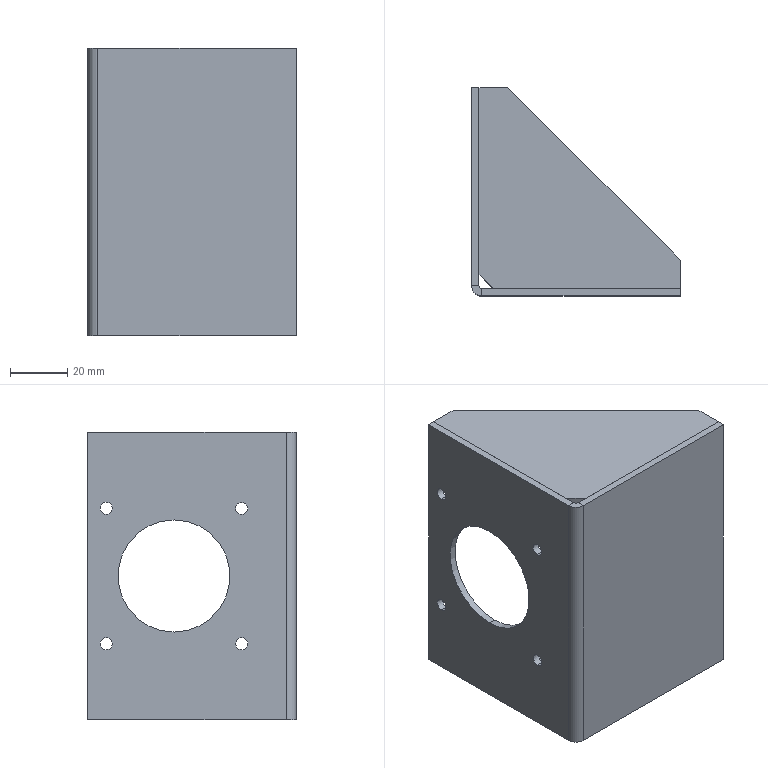Part | SolidWorks | features BaseBody 3 | 3 solids | 40 faces | box 72.5 x 72.5 x 100 mm | volume 47696 mm3 | plane 28 | cylinder 12 | commonest cylinder face diameters 4.2 x8 39 x2 2 x1 7 x1
STEP:
#1=CARTESIAN_POINT('',(0.,0.,50.));
#2=VERTEX_POINT('',#1);
#3=CARTESIAN_POINT('',(0.,-65.,50.));
#4=VERTEX_POINT('',#3);
#5=CARTESIAN_POINT('',(0.,-65.,50.));
#6=DIRECTION('',(0.,-1.,0.));
#7=VECTOR('',#6,1000.);
#8=LINE('',#5,#7);
#9=EDGE_CURVE('',#2,#4,#8,.T.);
#10=ORIENTED_EDGE('',*,*,#9,.T.);
#11=CARTESIAN_POINT('',(5.,-70.,50.));
#12=VERTEX_POINT('',#11);
#13=CARTESIAN_POINT('',(5.,-70.,50.));
#14=DIRECTION('',(0.7071,-0.7071,0.));
#15=VECTOR('',#14,1000.);
#16=LINE('',#13,#15);
#17=EDGE_CURVE('',#4,#12,#16,.T.);
#18=ORIENTED_EDGE('',*,*,#17,.T.);
#19=CARTESIAN_POINT('',(70.,-70.,50.));
#20=VERTEX_POINT('',#19);
#21=CARTESIAN_POINT('',(70.,-70.,50.));
#22=DIRECTION('',(1.,0.,0.));
#23=VECTOR('',#22,1000.);
#24=LINE('',#21,#23);
#25=EDGE_CURVE('',#12,#20,#24,.T.);
#26=ORIENTED_EDGE('',*,*,#25,.T.);
#27=CARTESIAN_POINT('',(70.,-60.,50.));
#28=VERTEX_POINT('',#27);
#29=CARTESIAN_POINT('',(70.,-60.,50.));
#30=DIRECTION('',(0.,1.,0.));
#31=VECTOR('',#30,1000.);
#32=LINE('',#29,#31);
#33=EDGE_CURVE('',#20,#28,#32,.T.);
#34=ORIENTED_EDGE('',*,*,#33,.T.);
#35=CARTESIAN_POINT('',(10.,0.,50.));
#36=VERTEX_POINT('',#35);
#37=CARTESIAN_POINT('',(10.,0.,50.));
#38=DIRECTION('',(-0.7071,0.7071,0.));
#39=VECTOR('',#38,1000.);
#40=LINE('',#37,#39);
#41=EDGE_CURVE('',#28,#36,#40,.T.);
#42=ORIENTED_EDGE('',*,*,#41,.T.);
#43=CARTESIAN_POINT('',(0.,0.,50.));
#44=DIRECTION('',(-1.,0.,0.));
#45=VECTOR('',#44,1000.);
#46=LINE('',#43,#45);
#47=EDGE_CURVE('',#36,#2,#46,.T.);
#48=ORIENTED_EDGE('',*,*,#47,.T.);
#49=EDGE_LOOP('',(#10,#18,#26,#34,#42,#48));
#50=FACE_OUTER_BOUND('',#49,.T.);
#51=CARTESIAN_POINT('',(0.,0.,50.));
#52=DIRECTION('',(0.,0.,-1.));
#53=DIRECTION('',(0.,-1.,0.));
#54=AXIS2_PLACEMENT_3D('',#51,#52,#53);
#55=PLANE('',#54);
#56=ADVANCED_FACE('',(#50),#55,.F.);
#57=CARTESIAN_POINT('',(0.,0.,47.5));
#58=VERTEX_POINT('',#57);
#59=CARTESIAN_POINT('',(0.,-65.,47.5));
#60=VERTEX_POINT('',#59);
#61=CARTESIAN_POINT('',(0.,-65.,47.5));
#62=DIRECTION('',(0.,-1.,0.));
#63=VECTOR('',#62,1000.);
#64=LINE('',#61,#63);
#65=EDGE_CURVE('',#58,#60,#64,.T.);
#66=ORIENTED_EDGE('',*,*,#65,.F.);
#67=CARTESIAN_POINT('',(10.,0.,47.5));
#68=VERTEX_POINT('',#67);
#69=CARTESIAN_POINT('',(0.,0.,47.5));
#70=DIRECTION('',(-1.,0.,0.));
#71=VECTOR('',#70,1000.);
#72=LINE('',#69,#71);
#73=EDGE_CURVE('',#68,#58,#72,.T.);
#74=ORIENTED_EDGE('',*,*,#73,.F.);
#75=CARTESIAN_POINT('',(70.,-60.,47.5));
#76=VERTEX_POINT('',#75);
#77=CARTESIAN_POINT('',(10.,0.,47.5));
#78=DIRECTION('',(-0.7071,0.7071,0.));
#79=VECTOR('',#78,1000.);
#80=LINE('',#77,#79);
#81=EDGE_CURVE('',#76,#68,#80,.T.);
#82=ORIENTED_EDGE('',*,*,#81,.F.);
#83=CARTESIAN_POINT('',(70.,-70.,47.5));
#84=VERTEX_POINT('',#83);
#85=CARTESIAN_POINT('',(70.,-60.,47.5));
#86=DIRECTION('',(0.,1.,0.));
#87=VECTOR('',#86,1000.);
#88=LINE('',#85,#87);
#89=EDGE_CURVE('',#84,#76,#88,.T.);
#90=ORIENTED_EDGE('',*,*,#89,.F.);
#91=CARTESIAN_POINT('',(5.,-70.,47.5));
#92=VERTEX_POINT('',#91);
#93=CARTESIAN_POINT('',(70.,-70.,47.5));
#94=DIRECTION('',(1.,0.,0.));
#95=VECTOR('',#94,1000.);
#96=LINE('',#93,#95);
#97=EDGE_CURVE('',#92,#84,#96,.T.);
#98=ORIENTED_EDGE('',*,*,#97,.F.);
#99=CARTESIAN_POINT('',(5.,-70.,47.5));
#100=DIRECTION('',(0.7071,-0.7071,0.));
#101=VECTOR('',#100,1000.);
#102=LINE('',#99,#101);
#103=EDGE_CURVE('',#60,#92,#102,.T.);
#104=ORIENTED_EDGE('',*,*,#103,.F.);
#105=EDGE_LOOP('',(#66,#74,#82,#90,#98,#104));
#106=FACE_OUTER_BOUND('',#105,.T.);
#107=CARTESIAN_POINT('',(0.,0.,47.5));
#108=DIRECTION('',(0.,0.,-1.));
#109=DIRECTION('',(0.,-1.,0.));
#110=AXIS2_PLACEMENT_3D('',#107,#108,#109);
#111=PLANE('',#110);
#112=ADVANCED_FACE('',(#106),#111,.T.);
#113=ORIENTED_EDGE('',*,*,#17,.F.);
#114=CARTESIAN_POINT('',(0.,-65.,47.5));
#115=DIRECTION('',(0.,0.,1.));
#116=VECTOR('',#115,1000.);
#117=LINE('',#114,#116);
#118=EDGE_CURVE('',#60,#4,#117,.T.);
#119=ORIENTED_EDGE('',*,*,#118,.F.);
#120=ORIENTED_EDGE('',*,*,#103,.T.);
#121=CARTESIAN_POINT('',(5.,-70.,47.5));
#122=DIRECTION('',(0.,0.,1.));
#123=VECTOR('',#122,1000.);
#124=LINE('',#121,#123);
#125=EDGE_CURVE('',#92,#12,#124,.T.);
#126=ORIENTED_EDGE('',*,*,#125,.T.);
#127=EDGE_LOOP('',(#113,#119,#120,#126));
#128=FACE_OUTER_BOUND('',#127,.T.);
#129=CARTESIAN_POINT('',(5.,-70.,47.5));
#130=DIRECTION('',(-0.7071,-0.7071,0.));
#131=DIRECTION('',(-0.7071,0.7071,0.));
#132=AXIS2_PLACEMENT_3D('',#129,#130,#131);
#133=PLANE('',#132);
#134=ADVANCED_FACE('',(#128),#133,.T.);
#135=ORIENTED_EDGE('',*,*,#25,.F.);
#136=ORIENTED_EDGE('',*,*,#125,.F.);
#137=ORIENTED_EDGE('',*,*,#97,.T.);
#138=CARTESIAN_POINT('',(70.,-70.,47.5));
#139=DIRECTION('',(0.,0.,1.));
#140=VECTOR('',#139,1000.);
#141=LINE('',#138,#140);
#142=EDGE_CURVE('',#84,#20,#141,.T.);
#143=ORIENTED_EDGE('',*,*,#142,.T.);
#144=EDGE_LOOP('',(#135,#136,#137,#143));
#145=FACE_OUTER_BOUND('',#144,.T.);
#146=CARTESIAN_POINT('',(70.,-70.,47.5));
#147=DIRECTION('',(0.,-1.,0.));
#148=DIRECTION('',(0.,0.,-1.));
#149=AXIS2_PLACEMENT_3D('',#146,#147,#148);
#150=PLANE('',#149);
#151=ADVANCED_FACE('',(#145),#150,.T.);
#152=ORIENTED_EDGE('',*,*,#33,.F.);
#153=ORIENTED_EDGE('',*,*,#142,.F.);
#154=ORIENTED_EDGE('',*,*,#89,.T.);
#155=CARTESIAN_POINT('',(70.,-60.,47.5));
#156=DIRECTION('',(0.,0.,1.));
#157=VECTOR('',#156,1000.);
#158=LINE('',#155,#157);
#159=EDGE_CURVE('',#76,#28,#158,.T.);
#160=ORIENTED_EDGE('',*,*,#159,.T.);
#161=EDGE_LOOP('',(#152,#153,#154,#160));
#162=FACE_OUTER_BOUND('',#161,.T.);
#163=CARTESIAN_POINT('',(70.,-60.,47.5));
#164=DIRECTION('',(1.,0.,0.));
#165=DIRECTION('',(0.,1.,0.));
#166=AXIS2_PLACEMENT_3D('',#163,#164,#165);
#167=PLANE('',#166);
#168=ADVANCED_FACE('',(#162),#167,.T.);
#169=ORIENTED_EDGE('',*,*,#41,.F.);
#170=ORIENTED_EDGE('',*,*,#159,.F.);
#171=ORIENTED_EDGE('',*,*,#81,.T.);
#172=CARTESIAN_POINT('',(10.,0.,47.5));
#173=DIRECTION('',(0.,0.,1.));
#174=VECTOR('',#173,1000.);
#175=LINE('',#172,#174);
#176=EDGE_CURVE('',#68,#36,#175,.T.);
#177=ORIENTED_EDGE('',*,*,#176,.T.);
#178=EDGE_LOOP('',(#169,#170,#171,#177));
#179=FACE_OUTER_BOUND('',#178,.T.);
#180=CARTESIAN_POINT('',(10.,0.,47.5));
#181=DIRECTION('',(0.7071,0.7071,0.));
#182=DIRECTION('',(0.,0.,-1.));
#183=AXIS2_PLACEMENT_3D('',#180,#181,#182);
#184=PLANE('',#183);
#185=ADVANCED_FACE('',(#179),#184,.T.);
#186=ORIENTED_EDGE('',*,*,#47,.F.);
#187=ORIENTED_EDGE('',*,*,#176,.F.);
#188=ORIENTED_EDGE('',*,*,#73,.T.);
#189=CARTESIAN_POINT('',(0.,0.,47.5));
#190=DIRECTION('',(0.,0.,1.));
#191=VECTOR('',#190,1000.);
#192=LINE('',#189,#191);
#193=EDGE_CURVE('',#58,#2,#192,.T.);
#194=ORIENTED_EDGE('',*,*,#193,.T.);
#195=EDGE_LOOP('',(#186,#187,#188,#194));
#196=FACE_OUTER_BOUND('',#195,.T.);
#197=CARTESIAN_POINT('',(0.,0.,47.5));
#198=DIRECTION('',(0.,1.,0.));
#199=DIRECTION('',(1.,0.,0.));
#200=AXIS2_PLACEMENT_3D('',#197,#198,#199);
#201=PLANE('',#200);
#202=ADVANCED_FACE('',(#196),#201,.T.);
#203=ORIENTED_EDGE('',*,*,#9,.F.);
#204=ORIENTED_EDGE('',*,*,#193,.F.);
#205=ORIENTED_EDGE('',*,*,#65,.T.);
#206=ORIENTED_EDGE('',*,*,#118,.T.);
#207=EDGE_LOOP('',(#203,#204,#205,#206));
#208=FACE_OUTER_BOUND('',#207,.T.);
#209=CARTESIAN_POINT('',(0.,-65.,47.5));
#210=DIRECTION('',(-1.,0.,0.));
#211=DIRECTION('',(0.,0.,1.));
#212=AXIS2_PLACEMENT_3D('',#209,#210,#211);
#213=PLANE('',#212);
#214=ADVANCED_FACE('',(#208),#213,.T.);
#215=CLOSED_SHELL('',(#56,#112,#134,#151,#168,#185,#202,#214));
#216=MANIFOLD_SOLID_BREP('',#215);
#217=CARTESIAN_POINT('',(0.,0.,-50.));
#218=VERTEX_POINT('',#217);
#219=CARTESIAN_POINT('',(0.,-65.,-50.));
#220=VERTEX_POINT('',#219);
#221=CARTESIAN_POINT('',(0.,-65.,-50.));
#222=DIRECTION('',(0.,-1.,0.));
#223=VECTOR('',#222,1000.);
#224=LINE('',#221,#223);
#225=EDGE_CURVE('',#218,#220,#224,.T.);
#226=ORIENTED_EDGE('',*,*,#225,.F.);
#227=CARTESIAN_POINT('',(10.,0.,-50.));
#228=VERTEX_POINT('',#227);
#229=CARTESIAN_POINT('',(0.,0.,-50.));
#230=DIRECTION('',(-1.,0.,0.));
#231=VECTOR('',#230,1000.);
#232=LINE('',#229,#231);
#233=EDGE_CURVE('',#228,#218,#232,.T.);
#234=ORIENTED_EDGE('',*,*,#233,.F.);
#235=CARTESIAN_POINT('',(70.,-60.,-50.));
#236=VERTEX_POINT('',#235);
#237=CARTESIAN_POINT('',(10.,0.,-50.));
#238=DIRECTION('',(-0.7071,0.7071,0.));
#239=VECTOR('',#238,1000.);
#240=LINE('',#237,#239);
#241=EDGE_CURVE('',#236,#228,#240,.T.);
#242=ORIENTED_EDGE('',*,*,#241,.F.);
#243=CARTESIAN_POINT('',(70.,-70.,-50.));
#244=VERTEX_POINT('',#243);
#245=CARTESIAN_POINT('',(70.,-60.,-50.));
#246=DIRECTION('',(0.,1.,0.));
#247=VECTOR('',#246,1000.);
#248=LINE('',#245,#247);
#249=EDGE_CURVE('',#244,#236,#248,.T.);
#250=ORIENTED_EDGE('',*,*,#249,.F.);
#251=CARTESIAN_POINT('',(5.,-70.,-50.));
#252=VERTEX_POINT('',#251);
#253=CARTESIAN_POINT('',(70.,-70.,-50.));
#254=DIRECTION('',(1.,0.,0.));
#255=VECTOR('',#254,1000.);
#256=LINE('',#253,#255);
#257=EDGE_CURVE('',#252,#244,#256,.T.);
#258=ORIENTED_EDGE('',*,*,#257,.F.);
#259=CARTESIAN_POINT('',(5.,-70.,-50.));
#260=DIRECTION('',(0.7071,-0.7071,0.));
#261=VECTOR('',#260,1000.);
#262=LINE('',#259,#261);
#263=EDGE_CURVE('',#220,#252,#262,.T.);
#264=ORIENTED_EDGE('',*,*,#263,.F.);
#265=EDGE_LOOP('',(#226,#234,#242,#250,#258,#264));
#266=FACE_OUTER_BOUND('',#265,.T.);
#267=CARTESIAN_POINT('',(0.,0.,-50.));
#268=DIRECTION('',(0.,0.,1.));
#269=DIRECTION('',(1.,0.,0.));
#270=AXIS2_PLACEMENT_3D('',#267,#268,#269);
#271=PLANE('',#270);
#272=ADVANCED_FACE('',(#266),#271,.F.);
#273=CARTESIAN_POINT('',(0.,0.,-47.5));
#274=VERTEX_POINT('',#273);
#275=CARTESIAN_POINT('',(0.,-65.,-47.5));
#276=VERTEX_POINT('',#275);
#277=CARTESIAN_POINT('',(0.,-65.,-47.5));
#278=DIRECTION('',(0.,-1.,0.));
#279=VECTOR('',#278,1000.);
#280=LINE('',#277,#279);
#281=EDGE_CURVE('',#274,#276,#280,.T.);
#282=ORIENTED_EDGE('',*,*,#281,.T.);
#283=CARTESIAN_POINT('',(5.,-70.,-47.5));
#284=VERTEX_POINT('',#283);
#285=CARTESIAN_POINT('',(5.,-70.,-47.5));
#286=DIRECTION('',(0.7071,-0.7071,0.));
#287=VECTOR('',#286,1000.);
#288=LINE('',#285,#287);
#289=EDGE_CURVE('',#276,#284,#288,.T.);
#290=ORIENTED_EDGE('',*,*,#289,.T.);
#291=CARTESIAN_POINT('',(70.,-70.,-47.5));
#292=VERTEX_POINT('',#291);
#293=CARTESIAN_POINT('',(70.,-70.,-47.5));
#294=DIRECTION('',(1.,0.,0.));
#295=VECTOR('',#294,1000.);
#296=LINE('',#293,#295);
#297=EDGE_CURVE('',#284,#292,#296,.T.);
#298=ORIENTED_EDGE('',*,*,#297,.T.);
#299=CARTESIAN_POINT('',(70.,-60.,-47.5));
#300=VERTEX_POINT('',#299);
#301=CARTESIAN_POINT('',(70.,-60.,-47.5));
#302=DIRECTION('',(0.,1.,0.));
#303=VECTOR('',#302,1000.);
#304=LINE('',#301,#303);
#305=EDGE_CURVE('',#292,#300,#304,.T.);
#306=ORIENTED_EDGE('',*,*,#305,.T.);
#307=CARTESIAN_POINT('',(10.,0.,-47.5));
#308=VERTEX_POINT('',#307);
#309=CARTESIAN_POINT('',(10.,0.,-47.5));
#310=DIRECTION('',(-0.7071,0.7071,0.));
#311=VECTOR('',#310,1000.);
#312=LINE('',#309,#311);
#313=EDGE_CURVE('',#300,#308,#312,.T.);
#314=ORIENTED_EDGE('',*,*,#313,.T.);
#315=CARTESIAN_POINT('',(0.,0.,-47.5));
#316=DIRECTION('',(-1.,0.,0.));
#317=VECTOR('',#316,1000.);
#318=LINE('',#315,#317);
#319=EDGE_CURVE('',#308,#274,#318,.T.);
#320=ORIENTED_EDGE('',*,*,#319,.T.);
#321=EDGE_LOOP('',(#282,#290,#298,#306,#314,#320));
#322=FACE_OUTER_BOUND('',#321,.T.);
#323=CARTESIAN_POINT('',(0.,0.,-47.5));
#324=DIRECTION('',(0.,0.,1.));
#325=DIRECTION('',(1.,0.,0.));
#326=AXIS2_PLACEMENT_3D('',#323,#324,#325);
#327=PLANE('',#326);
#328=ADVANCED_FACE('',(#322),#327,.T.);
#329=ORIENTED_EDGE('',*,*,#263,.T.);
#330=CARTESIAN_POINT('',(5.,-70.,-47.5));
#331=DIRECTION('',(0.,0.,-1.));
#332=VECTOR('',#331,1000.);
#333=LINE('',#330,#332);
#334=EDGE_CURVE('',#284,#252,#333,.T.);
#335=ORIENTED_EDGE('',*,*,#334,.F.);
#336=ORIENTED_EDGE('',*,*,#289,.F.);
#337=CARTESIAN_POINT('',(0.,-65.,-47.5));
#338=DIRECTION('',(0.,0.,-1.));
#339=VECTOR('',#338,1000.);
#340=LINE('',#337,#339);
#341=EDGE_CURVE('',#276,#220,#340,.T.);
#342=ORIENTED_EDGE('',*,*,#341,.T.);
#343=EDGE_LOOP('',(#329,#335,#336,#342));
#344=FACE_OUTER_BOUND('',#343,.T.);
#345=CARTESIAN_POINT('',(5.,-70.,-47.5));
#346=DIRECTION('',(-0.7071,-0.7071,0.));
#347=DIRECTION('',(-0.7071,0.7071,0.));
#348=AXIS2_PLACEMENT_3D('',#345,#346,#347);
#349=PLANE('',#348);
#350=ADVANCED_FACE('',(#344),#349,.T.);
#351=ORIENTED_EDGE('',*,*,#257,.T.);
#352=CARTESIAN_POINT('',(70.,-70.,-47.5));
#353=DIRECTION('',(0.,0.,-1.));
#354=VECTOR('',#353,1000.);
#355=LINE('',#352,#354);
#356=EDGE_CURVE('',#292,#244,#355,.T.);
#357=ORIENTED_EDGE('',*,*,#356,.F.);
#358=ORIENTED_EDGE('',*,*,#297,.F.);
#359=ORIENTED_EDGE('',*,*,#334,.T.);
#360=EDGE_LOOP('',(#351,#357,#358,#359));
#361=FACE_OUTER_BOUND('',#360,.T.);
#362=CARTESIAN_POINT('',(70.,-70.,-47.5));
#363=DIRECTION('',(0.,-1.,0.));
#364=DIRECTION('',(0.,0.,-1.));
#365=AXIS2_PLACEMENT_3D('',#362,#363,#364);
#366=PLANE('',#365);
#367=ADVANCED_FACE('',(#361),#366,.T.);
#368=ORIENTED_EDGE('',*,*,#249,.T.);
#369=CARTESIAN_POINT('',(70.,-60.,-47.5));
#370=DIRECTION('',(0.,0.,-1.));
#371=VECTOR('',#370,1000.);
#372=LINE('',#369,#371);
#373=EDGE_CURVE('',#300,#236,#372,.T.);
#374=ORIENTED_EDGE('',*,*,#373,.F.);
#375=ORIENTED_EDGE('',*,*,#305,.F.);
#376=ORIENTED_EDGE('',*,*,#356,.T.);
#377=EDGE_LOOP('',(#368,#374,#375,#376));
#378=FACE_OUTER_BOUND('',#377,.T.);
#379=CARTESIAN_POINT('',(70.,-60.,-47.5));
#380=DIRECTION('',(1.,0.,0.));
#381=DIRECTION('',(0.,1.,0.));
#382=AXIS2_PLACEMENT_3D('',#379,#380,#381);
#383=PLANE('',#382);
#384=ADVANCED_FACE('',(#378),#383,.T.);
#385=ORIENTED_EDGE('',*,*,#241,.T.);
#386=CARTESIAN_POINT('',(10.,0.,-47.5));
#387=DIRECTION('',(0.,0.,-1.));
#388=VECTOR('',#387,1000.);
#389=LINE('',#386,#388);
#390=EDGE_CURVE('',#308,#228,#389,.T.);
#391=ORIENTED_EDGE('',*,*,#390,.F.);
#392=ORIENTED_EDGE('',*,*,#313,.F.);
#393=ORIENTED_EDGE('',*,*,#373,.T.);
#394=EDGE_LOOP('',(#385,#391,#392,#393));
#395=FACE_OUTER_BOUND('',#394,.T.);
#396=CARTESIAN_POINT('',(10.,0.,-47.5));
#397=DIRECTION('',(0.7071,0.7071,0.));
#398=DIRECTION('',(0.,0.,-1.));
#399=AXIS2_PLACEMENT_3D('',#396,#397,#398);
#400=PLANE('',#399);
#401=ADVANCED_FACE('',(#395),#400,.T.);
#402=ORIENTED_EDGE('',*,*,#233,.T.);
#403=CARTESIAN_POINT('',(0.,0.,-47.5));
#404=DIRECTION('',(0.,0.,-1.));
#405=VECTOR('',#404,1000.);
#406=LINE('',#403,#405);
#407=EDGE_CURVE('',#274,#218,#406,.T.);
#408=ORIENTED_EDGE('',*,*,#407,.F.);
#409=ORIENTED_EDGE('',*,*,#319,.F.);
#410=ORIENTED_EDGE('',*,*,#390,.T.);
#411=EDGE_LOOP('',(#402,#408,#409,#410));
#412=FACE_OUTER_BOUND('',#411,.T.);
#413=CARTESIAN_POINT('',(0.,0.,-47.5));
#414=DIRECTION('',(0.,1.,0.));
#415=DIRECTION('',(1.,0.,0.));
#416=AXIS2_PLACEMENT_3D('',#413,#414,#415);
#417=PLANE('',#416);
#418=ADVANCED_FACE('',(#412),#417,.T.);
#419=ORIENTED_EDGE('',*,*,#225,.T.);
#420=ORIENTED_EDGE('',*,*,#341,.F.);
#421=ORIENTED_EDGE('',*,*,#281,.F.);
#422=ORIENTED_EDGE('',*,*,#407,.T.);
#423=EDGE_LOOP('',(#419,#420,#421,#422));
#424=FACE_OUTER_BOUND('',#423,.T.);
#425=CARTESIAN_POINT('',(0.,-65.,-47.5));
#426=DIRECTION('',(-1.,0.,0.));
#427=DIRECTION('',(0.,0.,1.));
#428=AXIS2_PLACEMENT_3D('',#425,#426,#427);
#429=PLANE('',#428);
#430=ADVANCED_FACE('',(#424),#429,.T.);
#431=CLOSED_SHELL('',(#272,#328,#350,#367,#384,#401,#418,#430));
#432=MANIFOLD_SOLID_BREP('',#431);
#433=CARTESIAN_POINT('',(0.,-53.57,-25.67));
#434=VERTEX_POINT('',#433);
#435=CARTESIAN_POINT('',(-2.5,-53.57,-25.67));
#436=VERTEX_POINT('',#435);
#437=CARTESIAN_POINT('',(-2.5,-53.57,-25.67));
#438=DIRECTION('',(-1.,0.,0.));
#439=VECTOR('',#438,1000.);
#440=LINE('',#437,#439);
#441=EDGE_CURVE('',#434,#436,#440,.T.);
#442=ORIENTED_EDGE('',*,*,#441,.F.);
#443=CARTESIAN_POINT('',(0.,-53.57,-21.47));
#444=VERTEX_POINT('',#443);
#445=CARTESIAN_POINT('',(0.,-53.57,-23.57));
#446=DIRECTION('',(1.,0.,0.));
#447=DIRECTION('',(0.,1.,0.));
#448=AXIS2_PLACEMENT_3D('',#445,#446,#447);
#449=CIRCLE('',#448,2.1);
#450=EDGE_CURVE('',#434,#444,#449,.T.);
#451=ORIENTED_EDGE('',*,*,#450,.T.);
#452=CARTESIAN_POINT('',(-2.5,-53.57,-21.47));
#453=VERTEX_POINT('',#452);
#454=CARTESIAN_POINT('',(-2.5,-53.57,-21.47));
#455=DIRECTION('',(-1.,0.,0.));
#456=VECTOR('',#455,1000.);
#457=LINE('',#454,#456);
#458=EDGE_CURVE('',#444,#453,#457,.T.);
#459=ORIENTED_EDGE('',*,*,#458,.T.);
#460=CARTESIAN_POINT('',(-2.5,-53.57,-23.57));
#461=DIRECTION('',(-1.,0.,0.));
#462=DIRECTION('',(0.,0.,1.));
#463=AXIS2_PLACEMENT_3D('',#460,#461,#462);
#464=CIRCLE('',#463,2.1);
#465=EDGE_CURVE('',#453,#436,#464,.T.);
#466=ORIENTED_EDGE('',*,*,#465,.T.);
#467=EDGE_LOOP('',(#442,#451,#459,#466));
#468=FACE_OUTER_BOUND('',#467,.T.);
#469=CARTESIAN_POINT('',(-2.5,-53.57,-23.57));
#470=DIRECTION('',(-1.,0.,0.));
#471=DIRECTION('',(0.,0.,1.));
#472=AXIS2_PLACEMENT_3D('',#469,#470,#471);
#473=CYLINDRICAL_SURFACE('',#472,2.1);
#474=ADVANCED_FACE('',(#468),#473,.F.);
#475=CARTESIAN_POINT('',(0.,-6.43,-25.67));
#476=VERTEX_POINT('',#475);
#477=CARTESIAN_POINT('',(-2.5,-6.43,-25.67));
#478=VERTEX_POINT('',#477);
#479=CARTESIAN_POINT('',(-2.5,-6.43,-25.67));
#480=DIRECTION('',(-1.,0.,0.));
#481=VECTOR('',#480,1000.);
#482=LINE('',#479,#481);
#483=EDGE_CURVE('',#476,#478,#482,.T.);
#484=ORIENTED_EDGE('',*,*,#483,.F.);
#485=CARTESIAN_POINT('',(0.,-6.43,-21.47));
#486=VERTEX_POINT('',#485);
#487=CARTESIAN_POINT('',(0.,-6.43,-23.57));
#488=DIRECTION('',(1.,0.,0.));
#489=DIRECTION('',(0.,1.,0.));
#490=AXIS2_PLACEMENT_3D('',#487,#488,#489);
#491=CIRCLE('',#490,2.1);
#492=EDGE_CURVE('',#476,#486,#491,.T.);
#493=ORIENTED_EDGE('',*,*,#492,.T.);
#494=CARTESIAN_POINT('',(-2.5,-6.43,-21.47));
#495=VERTEX_POINT('',#494);
#496=CARTESIAN_POINT('',(-2.5,-6.43,-21.47));
#497=DIRECTION('',(-1.,0.,0.));
#498=VECTOR('',#497,1000.);
#499=LINE('',#496,#498);
#500=EDGE_CURVE('',#486,#495,#499,.T.);
#501=ORIENTED_EDGE('',*,*,#500,.T.);
#502=CARTESIAN_POINT('',(-2.5,-6.43,-23.57));
#503=DIRECTION('',(-1.,0.,0.));
#504=DIRECTION('',(0.,0.,1.));
#505=AXIS2_PLACEMENT_3D('',#502,#503,#504);
#506=CIRCLE('',#505,2.1);
#507=EDGE_CURVE('',#495,#478,#506,.T.);
#508=ORIENTED_EDGE('',*,*,#507,.T.);
#509=EDGE_LOOP('',(#484,#493,#501,#508));
#510=FACE_OUTER_BOUND('',#509,.T.);
#511=CARTESIAN_POINT('',(-2.5,-6.43,-23.57));
#512=DIRECTION('',(-1.,0.,0.));
#513=DIRECTION('',(0.,0.,1.));
#514=AXIS2_PLACEMENT_3D('',#511,#512,#513);
#515=CYLINDRICAL_SURFACE('',#514,2.1);
#516=ADVANCED_FACE('',(#510),#515,.F.);
#517=CARTESIAN_POINT('',(0.,-53.5,21.4));
#518=VERTEX_POINT('',#517);
#519=CARTESIAN_POINT('',(-2.5,-53.5,21.4));
#520=VERTEX_POINT('',#519);
#521=CARTESIAN_POINT('',(-2.5,-53.5,21.4));
#522=DIRECTION('',(-1.,0.,0.));
#523=VECTOR('',#522,1000.);
#524=LINE('',#521,#523);
#525=EDGE_CURVE('',#518,#520,#524,.T.);
#526=ORIENTED_EDGE('',*,*,#525,.F.);
#527=CARTESIAN_POINT('',(0.,-53.5,25.6));
#528=VERTEX_POINT('',#527);
#529=CARTESIAN_POINT('',(0.,-53.5,23.5));
#530=DIRECTION('',(1.,0.,0.));
#531=DIRECTION('',(0.,1.,0.));
#532=AXIS2_PLACEMENT_3D('',#529,#530,#531);
#533=CIRCLE('',#532,2.1);
#534=EDGE_CURVE('',#518,#528,#533,.T.);
#535=ORIENTED_EDGE('',*,*,#534,.T.);
#536=CARTESIAN_POINT('',(-2.5,-53.5,25.6));
#537=VERTEX_POINT('',#536);
#538=CARTESIAN_POINT('',(-2.5,-53.5,25.6));
#539=DIRECTION('',(-1.,0.,0.));
#540=VECTOR('',#539,1000.);
#541=LINE('',#538,#540);
#542=EDGE_CURVE('',#528,#537,#541,.T.);
#543=ORIENTED_EDGE('',*,*,#542,.T.);
#544=CARTESIAN_POINT('',(-2.5,-53.5,23.5));
#545=DIRECTION('',(-1.,0.,0.));
#546=DIRECTION('',(0.,0.,1.));
#547=AXIS2_PLACEMENT_3D('',#544,#545,#546);
#548=CIRCLE('',#547,2.1);
#549=EDGE_CURVE('',#537,#520,#548,.T.);
#550=ORIENTED_EDGE('',*,*,#549,.T.);
#551=EDGE_LOOP('',(#526,#535,#543,#550));
#552=FACE_OUTER_BOUND('',#551,.T.);
#553=CARTESIAN_POINT('',(-2.5,-53.5,23.5));
#554=DIRECTION('',(-1.,0.,0.));
#555=DIRECTION('',(0.,0.,1.));
#556=AXIS2_PLACEMENT_3D('',#553,#554,#555);
#557=CYLINDRICAL_SURFACE('',#556,2.1);
#558=ADVANCED_FACE('',(#552),#557,.F.);
#559=CARTESIAN_POINT('',(0.,-6.43,21.47));
#560=VERTEX_POINT('',#559);
#561=CARTESIAN_POINT('',(-2.5,-6.43,21.47));
#562=VERTEX_POINT('',#561);
#563=CARTESIAN_POINT('',(-2.5,-6.43,21.47));
#564=DIRECTION('',(-1.,0.,0.));
#565=VECTOR('',#564,1000.);
#566=LINE('',#563,#565);
#567=EDGE_CURVE('',#560,#562,#566,.T.);
#568=ORIENTED_EDGE('',*,*,#567,.F.);
#569=CARTESIAN_POINT('',(0.,-6.43,25.67));
#570=VERTEX_POINT('',#569);
#571=CARTESIAN_POINT('',(0.,-6.43,23.57));
#572=DIRECTION('',(1.,0.,0.));
#573=DIRECTION('',(0.,1.,0.));
#574=AXIS2_PLACEMENT_3D('',#571,#572,#573);
#575=CIRCLE('',#574,2.1);
#576=EDGE_CURVE('',#560,#570,#575,.T.);
#577=ORIENTED_EDGE('',*,*,#576,.T.);
#578=CARTESIAN_POINT('',(-2.5,-6.43,25.67));
#579=VERTEX_POINT('',#578);
#580=CARTESIAN_POINT('',(-2.5,-6.43,25.67));
#581=DIRECTION('',(-1.,0.,0.));
#582=VECTOR('',#581,1000.);
#583=LINE('',#580,#582);
#584=EDGE_CURVE('',#570,#579,#583,.T.);
#585=ORIENTED_EDGE('',*,*,#584,.T.);
#586=CARTESIAN_POINT('',(-2.5,-6.43,23.57));
#587=DIRECTION('',(-1.,0.,0.));
#588=DIRECTION('',(0.,0.,1.));
#589=AXIS2_PLACEMENT_3D('',#586,#587,#588);
#590=CIRCLE('',#589,2.1);
#591=EDGE_CURVE('',#579,#562,#590,.T.);
#592=ORIENTED_EDGE('',*,*,#591,.T.);
#593=EDGE_LOOP('',(#568,#577,#585,#592));
#594=FACE_OUTER_BOUND('',#593,.T.);
#595=CARTESIAN_POINT('',(-2.5,-6.43,23.57));
#596=DIRECTION('',(-1.,0.,0.));
#597=DIRECTION('',(0.,0.,1.));
#598=AXIS2_PLACEMENT_3D('',#595,#596,#597);
#599=CYLINDRICAL_SURFACE('',#598,2.1);
#600=ADVANCED_FACE('',(#594),#599,.F.);
#601=CARTESIAN_POINT('',(0.,-30.,-19.5));
#602=VERTEX_POINT('',#601);
#603=CARTESIAN_POINT('',(-2.5,-30.,-19.5));
#604=VERTEX_POINT('',#603);
#605=CARTESIAN_POINT('',(7.5,-30.,-19.5));
#606=DIRECTION('',(-1.,0.,0.));
#607=VECTOR('',#606,1000.);
#608=LINE('',#605,#607);
#609=EDGE_CURVE('',#602,#604,#608,.T.);
#610=ORIENTED_EDGE('',*,*,#609,.F.);
#611=CARTESIAN_POINT('',(0.,-30.,19.5));
#612=VERTEX_POINT('',#611);
#613=CARTESIAN_POINT('',(0.,-30.,0.));
#614=DIRECTION('',(1.,0.,0.));
#615=DIRECTION('',(0.,1.,0.));
#616=AXIS2_PLACEMENT_3D('',#613,#614,#615);
#617=CIRCLE('',#616,19.5);
#618=EDGE_CURVE('',#602,#612,#617,.T.);
#619=ORIENTED_EDGE('',*,*,#618,.T.);
#620=CARTESIAN_POINT('',(-2.5,-30.,19.5));
#621=VERTEX_POINT('',#620);
#622=CARTESIAN_POINT('',(7.5,-30.,19.5));
#623=DIRECTION('',(-1.,0.,0.));
#624=VECTOR('',#623,1000.);
#625=LINE('',#622,#624);
#626=EDGE_CURVE('',#612,#621,#625,.T.);
#627=ORIENTED_EDGE('',*,*,#626,.T.);
#628=CARTESIAN_POINT('',(-2.5,-30.,0.));
#629=DIRECTION('',(-1.,0.,0.));
#630=DIRECTION('',(0.,0.,1.));
#631=AXIS2_PLACEMENT_3D('',#628,#629,#630);
#632=CIRCLE('',#631,19.5);
#633=EDGE_CURVE('',#621,#604,#632,.T.);
#634=ORIENTED_EDGE('',*,*,#633,.T.);
#635=EDGE_LOOP('',(#610,#619,#627,#634));
#636=FACE_OUTER_BOUND('',#635,.T.);
#637=CARTESIAN_POINT('',(7.5,-30.,0.));
#638=DIRECTION('',(-1.,0.,0.));
#639=DIRECTION('',(0.,0.,1.));
#640=AXIS2_PLACEMENT_3D('',#637,#638,#639);
#641=CYLINDRICAL_SURFACE('',#640,19.5);
#642=ADVANCED_FACE('',(#636),#641,.F.);
#643=CARTESIAN_POINT('',(1.,-72.5,-50.));
#644=VERTEX_POINT('',#643);
#645=CARTESIAN_POINT('',(70.,-72.5,-50.));
#646=VERTEX_POINT('',#645);
#647=CARTESIAN_POINT('',(0.,-72.5,-50.));
#648=DIRECTION('',(1.,0.,0.));
#649=VECTOR('',#648,1000.);
#650=LINE('',#647,#649);
#651=EDGE_CURVE('',#644,#646,#650,.T.);
#652=ORIENTED_EDGE('',*,*,#651,.F.);
#653=CARTESIAN_POINT('',(1.,-70.,-50.));
#654=VERTEX_POINT('',#653);
#655=CARTESIAN_POINT('',(1.,-72.5,-50.));
#656=DIRECTION('',(0.,1.,0.));
#657=VECTOR('',#656,1000.);
#658=LINE('',#655,#657);
#659=EDGE_CURVE('',#644,#654,#658,.T.);
#660=ORIENTED_EDGE('',*,*,#659,.T.);
#661=CARTESIAN_POINT('',(70.,-70.,-50.));
#662=VERTEX_POINT('',#661);
#663=CARTESIAN_POINT('',(0.,-70.,-50.));
#664=DIRECTION('',(1.,0.,0.));
#665=VECTOR('',#664,1000.);
#666=LINE('',#663,#665);
#667=EDGE_CURVE('',#654,#662,#666,.T.);
#668=ORIENTED_EDGE('',*,*,#667,.T.);
#669=CARTESIAN_POINT('',(70.,-70.,-50.));
#670=DIRECTION('',(0.,-1.,0.));
#671=VECTOR('',#670,1000.);
#672=LINE('',#669,#671);
#673=EDGE_CURVE('',#662,#646,#672,.T.);
#674=ORIENTED_EDGE('',*,*,#673,.T.);
#675=EDGE_LOOP('',(#652,#660,#668,#674));
#676=FACE_OUTER_BOUND('',#675,.T.);
#677=CARTESIAN_POINT('',(1.,-69.,-50.));
#678=DIRECTION('',(0.,0.,-1.));
#679=DIRECTION('',(0.,-1.,0.));
#680=AXIS2_PLACEMENT_3D('',#677,#678,#679);
#681=PLANE('',#680);
#682=ADVANCED_FACE('',(#676),#681,.T.);
#683=CARTESIAN_POINT('',(-2.5,0.,50.));
#684=VERTEX_POINT('',#683);
#685=CARTESIAN_POINT('',(-2.5,-69.,50.));
#686=VERTEX_POINT('',#685);
#687=CARTESIAN_POINT('',(-2.5,0.,50.));
#688=DIRECTION('',(0.,-1.,0.));
#689=VECTOR('',#688,1000.);
#690=LINE('',#687,#689);
#691=EDGE_CURVE('',#684,#686,#690,.T.);
#692=ORIENTED_EDGE('',*,*,#691,.T.);
#693=CARTESIAN_POINT('',(0.,-69.,50.));
#694=VERTEX_POINT('',#693);
#695=CARTESIAN_POINT('',(-2.5,-69.,50.));
#696=DIRECTION('',(1.,0.,0.));
#697=VECTOR('',#696,1000.);
#698=LINE('',#695,#697);
#699=EDGE_CURVE('',#686,#694,#698,.T.);
#700=ORIENTED_EDGE('',*,*,#699,.T.);
#701=CARTESIAN_POINT('',(0.,0.,50.));
#702=VERTEX_POINT('',#701);
#703=CARTESIAN_POINT('',(0.,0.,50.));
#704=DIRECTION('',(0.,-1.,0.));
#705=VECTOR('',#704,1000.);
#706=LINE('',#703,#705);
#707=EDGE_CURVE('',#702,#694,#706,.T.);
#708=ORIENTED_EDGE('',*,*,#707,.F.);
#709=CARTESIAN_POINT('',(-2.5,0.,50.));
#710=DIRECTION('',(1.,0.,0.));
#711=VECTOR('',#710,1000.);
#712=LINE('',#709,#711);
#713=EDGE_CURVE('',#684,#702,#712,.T.);
#714=ORIENTED_EDGE('',*,*,#713,.F.);
#715=EDGE_LOOP('',(#692,#700,#708,#714));
#716=FACE_OUTER_BOUND('',#715,.T.);
#717=CARTESIAN_POINT('',(1.,-69.,50.));
#718=DIRECTION('',(0.,0.,-1.));
#719=DIRECTION('',(0.,-1.,0.));
#720=AXIS2_PLACEMENT_3D('',#717,#718,#719);
#721=PLANE('',#720);
#722=ADVANCED_FACE('',(#716),#721,.F.);
#723=CARTESIAN_POINT('',(-2.5,-69.,-50.));
#724=VERTEX_POINT('',#723);
#725=CARTESIAN_POINT('',(1.,-69.,-50.));
#726=DIRECTION('',(0.,0.,1.));
#727=DIRECTION('',(1.,0.,0.));
#728=AXIS2_PLACEMENT_3D('',#725,#726,#727);
#729=CIRCLE('',#728,3.5);
#730=EDGE_CURVE('',#724,#644,#729,.T.);
#731=ORIENTED_EDGE('',*,*,#730,.T.);
#732=CARTESIAN_POINT('',(1.,-72.5,50.));
#733=VERTEX_POINT('',#732);
#734=CARTESIAN_POINT('',(1.,-72.5,50.));
#735=DIRECTION('',(0.,0.,-1.));
#736=VECTOR('',#735,1000.);
#737=LINE('',#734,#736);
#738=EDGE_CURVE('',#733,#644,#737,.T.);
#739=ORIENTED_EDGE('',*,*,#738,.F.);
#740=CARTESIAN_POINT('',(1.,-69.,50.));
#741=DIRECTION('',(0.,0.,1.));
#742=DIRECTION('',(1.,0.,0.));
#743=AXIS2_PLACEMENT_3D('',#740,#741,#742);
#744=CIRCLE('',#743,3.5);
#745=EDGE_CURVE('',#686,#733,#744,.T.);
#746=ORIENTED_EDGE('',*,*,#745,.F.);
#747=CARTESIAN_POINT('',(-2.5,-69.,50.));
#748=DIRECTION('',(0.,0.,-1.));
#749=VECTOR('',#748,1000.);
#750=LINE('',#747,#749);
#751=EDGE_CURVE('',#686,#724,#750,.T.);
#752=ORIENTED_EDGE('',*,*,#751,.T.);
#753=EDGE_LOOP('',(#731,#739,#746,#752));
#754=FACE_OUTER_BOUND('',#753,.T.);
#755=CARTESIAN_POINT('',(1.,-69.,50.));
#756=DIRECTION('',(0.,0.,-1.));
#757=DIRECTION('',(-1.,0.,0.));
#758=AXIS2_PLACEMENT_3D('',#755,#756,#757);
#759=CYLINDRICAL_SURFACE('',#758,3.5);
#760=ADVANCED_FACE('',(#754),#759,.T.);
#761=CARTESIAN_POINT('',(-2.5,0.,-50.));
#762=VERTEX_POINT('',#761);
#763=CARTESIAN_POINT('',(0.,0.,-50.));
#764=VERTEX_POINT('',#763);
#765=CARTESIAN_POINT('',(-2.5,0.,-50.));
#766=DIRECTION('',(1.,0.,0.));
#767=VECTOR('',#766,1000.);
#768=LINE('',#765,#767);
#769=EDGE_CURVE('',#762,#764,#768,.T.);
#770=ORIENTED_EDGE('',*,*,#769,.F.);
#771=CARTESIAN_POINT('',(-2.5,0.,50.));
#772=DIRECTION('',(0.,0.,-1.));
#773=VECTOR('',#772,1000.);
#774=LINE('',#771,#773);
#775=EDGE_CURVE('',#684,#762,#774,.T.);
#776=ORIENTED_EDGE('',*,*,#775,.F.);
#777=ORIENTED_EDGE('',*,*,#713,.T.);
#778=CARTESIAN_POINT('',(0.,0.,50.));
#779=DIRECTION('',(0.,0.,-1.));
#780=VECTOR('',#779,1000.);
#781=LINE('',#778,#780);
#782=EDGE_CURVE('',#702,#764,#781,.T.);
#783=ORIENTED_EDGE('',*,*,#782,.T.);
#784=EDGE_LOOP('',(#770,#776,#777,#783));
#785=FACE_OUTER_BOUND('',#784,.T.);
#786=CARTESIAN_POINT('',(-2.5,0.,50.));
#787=DIRECTION('',(0.,1.,0.));
#788=DIRECTION('',(1.,0.,0.));
#789=AXIS2_PLACEMENT_3D('',#786,#787,#788);
#790=PLANE('',#789);
#791=ADVANCED_FACE('',(#785),#790,.T.);
#792=CARTESIAN_POINT('',(0.,-30.,0.));
#793=DIRECTION('',(1.,0.,0.));
#794=DIRECTION('',(0.,1.,0.));
#795=AXIS2_PLACEMENT_3D('',#792,#793,#794);
#796=CIRCLE('',#795,19.5);
#797=EDGE_CURVE('',#612,#602,#796,.T.);
#798=ORIENTED_EDGE('',*,*,#797,.F.);
#799=ORIENTED_EDGE('',*,*,#618,.F.);
#800=EDGE_LOOP('',(#798,#799));
#801=FACE_BOUND('',#800,.T.);
#802=CARTESIAN_POINT('',(0.,-6.43,23.57));
#803=DIRECTION('',(1.,0.,0.));
#804=DIRECTION('',(0.,1.,0.));
#805=AXIS2_PLACEMENT_3D('',#802,#803,#804);
#806=CIRCLE('',#805,2.1);
#807=EDGE_CURVE('',#570,#560,#806,.T.);
#808=ORIENTED_EDGE('',*,*,#807,.F.);
#809=ORIENTED_EDGE('',*,*,#576,.F.);
#810=EDGE_LOOP('',(#808,#809));
#811=FACE_BOUND('',#810,.T.);
#812=CARTESIAN_POINT('',(0.,-53.5,23.5));
#813=DIRECTION('',(1.,0.,0.));
#814=DIRECTION('',(0.,1.,0.));
#815=AXIS2_PLACEMENT_3D('',#812,#813,#814);
#816=CIRCLE('',#815,2.1);
#817=EDGE_CURVE('',#528,#518,#816,.T.);
#818=ORIENTED_EDGE('',*,*,#817,.F.);
#819=ORIENTED_EDGE('',*,*,#534,.F.);
#820=EDGE_LOOP('',(#818,#819));
#821=FACE_BOUND('',#820,.T.);
#822=CARTESIAN_POINT('',(0.,-6.43,-23.57));
#823=DIRECTION('',(1.,0.,0.));
#824=DIRECTION('',(0.,1.,0.));
#825=AXIS2_PLACEMENT_3D('',#822,#823,#824);
#826=CIRCLE('',#825,2.1);
#827=EDGE_CURVE('',#486,#476,#826,.T.);
#828=ORIENTED_EDGE('',*,*,#827,.F.);
#829=ORIENTED_EDGE('',*,*,#492,.F.);
#830=EDGE_LOOP('',(#828,#829));
#831=FACE_BOUND('',#830,.T.);
#832=CARTESIAN_POINT('',(0.,-53.57,-23.57));
#833=DIRECTION('',(1.,0.,0.));
#834=DIRECTION('',(0.,1.,0.));
#835=AXIS2_PLACEMENT_3D('',#832,#833,#834);
#836=CIRCLE('',#835,2.1);
#837=EDGE_CURVE('',#444,#434,#836,.T.);
#838=ORIENTED_EDGE('',*,*,#837,.F.);
#839=ORIENTED_EDGE('',*,*,#450,.F.);
#840=EDGE_LOOP('',(#838,#839));
#841=FACE_BOUND('',#840,.T.);
#842=CARTESIAN_POINT('',(0.,-69.,-50.));
#843=VERTEX_POINT('',#842);
#844=CARTESIAN_POINT('',(0.,0.,-50.));
#845=DIRECTION('',(0.,-1.,0.));
#846=VECTOR('',#845,1000.);
#847=LINE('',#844,#846);
#848=EDGE_CURVE('',#764,#843,#847,.T.);
#849=ORIENTED_EDGE('',*,*,#848,.F.);
#850=ORIENTED_EDGE('',*,*,#782,.F.);
#851=ORIENTED_EDGE('',*,*,#707,.T.);
#852=CARTESIAN_POINT('',(0.,-69.,50.));
#853=DIRECTION('',(0.,0.,-1.));
#854=VECTOR('',#853,1000.);
#855=LINE('',#852,#854);
#856=EDGE_CURVE('',#694,#843,#855,.T.);
#857=ORIENTED_EDGE('',*,*,#856,.T.);
#858=EDGE_LOOP('',(#849,#850,#851,#857));
#859=FACE_OUTER_BOUND('',#858,.T.);
#860=CARTESIAN_POINT('',(0.,0.,50.));
#861=DIRECTION('',(1.,0.,0.));
#862=DIRECTION('',(0.,1.,0.));
#863=AXIS2_PLACEMENT_3D('',#860,#861,#862);
#864=PLANE('',#863);
#865=ADVANCED_FACE('',(#801,#811,#821,#831,#841,#859),#864,.T.);
#866=CARTESIAN_POINT('',(1.,-69.,-50.));
#867=DIRECTION('',(0.,0.,1.));
#868=DIRECTION('',(-1.,0.,0.));
#869=AXIS2_PLACEMENT_3D('',#866,#867,#868);
#870=CIRCLE('',#869,1.);
#871=EDGE_CURVE('',#843,#654,#870,.T.);
#872=ORIENTED_EDGE('',*,*,#871,.F.);
#873=ORIENTED_EDGE('',*,*,#856,.F.);
#874=CARTESIAN_POINT('',(1.,-70.,50.));
#875=VERTEX_POINT('',#874);
#876=CARTESIAN_POINT('',(1.,-69.,50.));
#877=DIRECTION('',(0.,0.,1.));
#878=DIRECTION('',(-1.,0.,0.));
#879=AXIS2_PLACEMENT_3D('',#876,#877,#878);
#880=CIRCLE('',#879,1.);
#881=EDGE_CURVE('',#694,#875,#880,.T.);
#882=ORIENTED_EDGE('',*,*,#881,.T.);
#883=CARTESIAN_POINT('',(1.,-70.,50.));
#884=DIRECTION('',(0.,0.,-1.));
#885=VECTOR('',#884,1000.);
#886=LINE('',#883,#885);
#887=EDGE_CURVE('',#875,#654,#886,.T.);
#888=ORIENTED_EDGE('',*,*,#887,.T.);
#889=EDGE_LOOP('',(#872,#873,#882,#888));
#890=FACE_OUTER_BOUND('',#889,.T.);
#891=CARTESIAN_POINT('',(1.,-69.,50.));
#892=DIRECTION('',(0.,0.,-1.));
#893=DIRECTION('',(-1.,0.,0.));
#894=AXIS2_PLACEMENT_3D('',#891,#892,#893);
#895=CYLINDRICAL_SURFACE('',#894,1.);
#896=ADVANCED_FACE('',(#890),#895,.F.);
#897=ORIENTED_EDGE('',*,*,#667,.F.);
#898=ORIENTED_EDGE('',*,*,#887,.F.);
#899=CARTESIAN_POINT('',(70.,-70.,50.));
#900=VERTEX_POINT('',#899);
#901=CARTESIAN_POINT('',(0.,-70.,50.));
#902=DIRECTION('',(1.,0.,0.));
#903=VECTOR('',#902,1000.);
#904=LINE('',#901,#903);
#905=EDGE_CURVE('',#875,#900,#904,.T.);
#906=ORIENTED_EDGE('',*,*,#905,.T.);
#907=CARTESIAN_POINT('',(70.,-70.,50.));
#908=DIRECTION('',(0.,0.,-1.));
#909=VECTOR('',#908,1000.);
#910=LINE('',#907,#909);
#911=EDGE_CURVE('',#900,#662,#910,.T.);
#912=ORIENTED_EDGE('',*,*,#911,.T.);
#913=EDGE_LOOP('',(#897,#898,#906,#912));
#914=FACE_OUTER_BOUND('',#913,.T.);
#915=CARTESIAN_POINT('',(0.,-70.,50.));
#916=DIRECTION('',(0.,1.,0.));
#917=DIRECTION('',(1.,0.,0.));
#918=AXIS2_PLACEMENT_3D('',#915,#916,#917);
#919=PLANE('',#918);
#920=ADVANCED_FACE('',(#914),#919,.T.);
#921=ORIENTED_EDGE('',*,*,#673,.F.);
#922=ORIENTED_EDGE('',*,*,#911,.F.);
#923=CARTESIAN_POINT('',(70.,-72.5,50.));
#924=VERTEX_POINT('',#923);
#925=CARTESIAN_POINT('',(70.,-70.,50.));
#926=DIRECTION('',(0.,-1.,0.));
#927=VECTOR('',#926,1000.);
#928=LINE('',#925,#927);
#929=EDGE_CURVE('',#900,#924,#928,.T.);
#930=ORIENTED_EDGE('',*,*,#929,.T.);
#931=CARTESIAN_POINT('',(70.,-72.5,50.));
#932=DIRECTION('',(0.,0.,-1.));
#933=VECTOR('',#932,1000.);
#934=LINE('',#931,#933);
#935=EDGE_CURVE('',#924,#646,#934,.T.);
#936=ORIENTED_EDGE('',*,*,#935,.T.);
#937=EDGE_LOOP('',(#921,#922,#930,#936));
#938=FACE_OUTER_BOUND('',#937,.T.);
#939=CARTESIAN_POINT('',(70.,-70.,50.));
#940=DIRECTION('',(1.,0.,0.));
#941=DIRECTION('',(0.,1.,0.));
#942=AXIS2_PLACEMENT_3D('',#939,#940,#941);
#943=PLANE('',#942);
#944=ADVANCED_FACE('',(#938),#943,.T.);
#945=ORIENTED_EDGE('',*,*,#651,.T.);
#946=ORIENTED_EDGE('',*,*,#935,.F.);
#947=CARTESIAN_POINT('',(0.,-72.5,50.));
#948=DIRECTION('',(1.,0.,0.));
#949=VECTOR('',#948,1000.);
#950=LINE('',#947,#949);
#951=EDGE_CURVE('',#733,#924,#950,.T.);
#952=ORIENTED_EDGE('',*,*,#951,.F.);
#953=ORIENTED_EDGE('',*,*,#738,.T.);
#954=EDGE_LOOP('',(#945,#946,#952,#953));
#955=FACE_OUTER_BOUND('',#954,.T.);
#956=CARTESIAN_POINT('',(0.,-72.5,50.));
#957=DIRECTION('',(0.,1.,0.));
#958=DIRECTION('',(1.,0.,0.));
#959=AXIS2_PLACEMENT_3D('',#956,#957,#958);
#960=PLANE('',#959);
#961=ADVANCED_FACE('',(#955),#960,.F.);
#962=ORIENTED_EDGE('',*,*,#848,.T.);
#963=CARTESIAN_POINT('',(0.,-69.,-50.));
#964=DIRECTION('',(-1.,0.,0.));
#965=VECTOR('',#964,1000.);
#966=LINE('',#963,#965);
#967=EDGE_CURVE('',#843,#724,#966,.T.);
#968=ORIENTED_EDGE('',*,*,#967,.T.);
#969=CARTESIAN_POINT('',(-2.5,0.,-50.));
#970=DIRECTION('',(0.,-1.,0.));
#971=VECTOR('',#970,1000.);
#972=LINE('',#969,#971);
#973=EDGE_CURVE('',#762,#724,#972,.T.);
#974=ORIENTED_EDGE('',*,*,#973,.F.);
#975=ORIENTED_EDGE('',*,*,#769,.T.);
#976=EDGE_LOOP('',(#962,#968,#974,#975));
#977=FACE_OUTER_BOUND('',#976,.T.);
#978=CARTESIAN_POINT('',(1.,-72.5,-50.));
#979=DIRECTION('',(0.,0.,-1.));
#980=DIRECTION('',(0.,-1.,0.));
#981=AXIS2_PLACEMENT_3D('',#978,#979,#980);
#982=PLANE('',#981);
#983=ADVANCED_FACE('',(#977),#982,.T.);
#984=ORIENTED_EDGE('',*,*,#967,.F.);
#985=ORIENTED_EDGE('',*,*,#871,.T.);
#986=ORIENTED_EDGE('',*,*,#659,.F.);
#987=ORIENTED_EDGE('',*,*,#730,.F.);
#988=EDGE_LOOP('',(#984,#985,#986,#987));
#989=FACE_OUTER_BOUND('',#988,.T.);
#990=CARTESIAN_POINT('',(0.,-69.,-50.));
#991=DIRECTION('',(0.,0.,-1.));
#992=DIRECTION('',(0.,-1.,0.));
#993=AXIS2_PLACEMENT_3D('',#990,#991,#992);
#994=PLANE('',#993);
#995=ADVANCED_FACE('',(#989),#994,.T.);
#996=ORIENTED_EDGE('',*,*,#905,.F.);
#997=CARTESIAN_POINT('',(1.,-70.,50.));
#998=DIRECTION('',(0.,-1.,0.));
#999=VECTOR('',#998,1000.);
#1000=LINE('',#997,#999);
#1001=EDGE_CURVE('',#875,#733,#1000,.T.);
#1002=ORIENTED_EDGE('',*,*,#1001,.T.);
#1003=ORIENTED_EDGE('',*,*,#951,.T.);
#1004=ORIENTED_EDGE('',*,*,#929,.F.);
#1005=EDGE_LOOP('',(#996,#1002,#1003,#1004));
#1006=FACE_OUTER_BOUND('',#1005,.T.);
#1007=CARTESIAN_POINT('',(-2.5,-69.,50.));
#1008=DIRECTION('',(0.,0.,1.));
#1009=DIRECTION('',(1.,0.,0.));
#1010=AXIS2_PLACEMENT_3D('',#1007,#1008,#1009);
#1011=PLANE('',#1010);
#1012=ADVANCED_FACE('',(#1006),#1011,.T.);
#1013=ORIENTED_EDGE('',*,*,#1001,.F.);
#1014=ORIENTED_EDGE('',*,*,#881,.F.);
#1015=ORIENTED_EDGE('',*,*,#699,.F.);
#1016=ORIENTED_EDGE('',*,*,#745,.T.);
#1017=EDGE_LOOP('',(#1013,#1014,#1015,#1016));
#1018=FACE_OUTER_BOUND('',#1017,.T.);
#1019=CARTESIAN_POINT('',(1.,-70.,50.));
#1020=DIRECTION('',(0.,0.,1.));
#1021=DIRECTION('',(1.,0.,0.));
#1022=AXIS2_PLACEMENT_3D('',#1019,#1020,#1021);
#1023=PLANE('',#1022);
#1024=ADVANCED_FACE('',(#1018),#1023,.T.);
#1025=ORIENTED_EDGE('',*,*,#549,.F.);
#1026=CARTESIAN_POINT('',(-2.5,-53.5,23.5));
#1027=DIRECTION('',(-1.,0.,0.));
#1028=DIRECTION('',(0.,0.,1.));
#1029=AXIS2_PLACEMENT_3D('',#1026,#1027,#1028);
#1030=CIRCLE('',#1029,2.1);
#1031=EDGE_CURVE('',#520,#537,#1030,.T.);
#1032=ORIENTED_EDGE('',*,*,#1031,.F.);
#1033=EDGE_LOOP('',(#1025,#1032));
#1034=FACE_BOUND('',#1033,.T.);
#1035=ORIENTED_EDGE('',*,*,#633,.F.);
#1036=CARTESIAN_POINT('',(-2.5,-30.,0.));
#1037=DIRECTION('',(-1.,0.,0.));
#1038=DIRECTION('',(0.,0.,1.));
#1039=AXIS2_PLACEMENT_3D('',#1036,#1037,#1038);
#1040=CIRCLE('',#1039,19.5);
#1041=EDGE_CURVE('',#604,#621,#1040,.T.);
#1042=ORIENTED_EDGE('',*,*,#1041,.F.);
#1043=EDGE_LOOP('',(#1035,#1042));
#1044=FACE_BOUND('',#1043,.T.);
#1045=ORIENTED_EDGE('',*,*,#591,.F.);
#1046=CARTESIAN_POINT('',(-2.5,-6.43,23.57));
#1047=DIRECTION('',(-1.,0.,0.));
#1048=DIRECTION('',(0.,0.,1.));
#1049=AXIS2_PLACEMENT_3D('',#1046,#1047,#1048);
#1050=CIRCLE('',#1049,2.1);
#1051=EDGE_CURVE('',#562,#579,#1050,.T.);
#1052=ORIENTED_EDGE('',*,*,#1051,.F.);
#1053=EDGE_LOOP('',(#1045,#1052));
#1054=FACE_BOUND('',#1053,.T.);
#1055=ORIENTED_EDGE('',*,*,#507,.F.);
#1056=CARTESIAN_POINT('',(-2.5,-6.43,-23.57));
#1057=DIRECTION('',(-1.,0.,0.));
#1058=DIRECTION('',(0.,0.,1.));
#1059=AXIS2_PLACEMENT_3D('',#1056,#1057,#1058);
#1060=CIRCLE('',#1059,2.1);
#1061=EDGE_CURVE('',#478,#495,#1060,.T.);
#1062=ORIENTED_EDGE('',*,*,#1061,.F.);
#1063=EDGE_LOOP('',(#1055,#1062));
#1064=FACE_BOUND('',#1063,.T.);
#1065=ORIENTED_EDGE('',*,*,#465,.F.);
#1066=CARTESIAN_POINT('',(-2.5,-53.57,-23.57));
#1067=DIRECTION('',(-1.,0.,0.));
#1068=DIRECTION('',(0.,0.,1.));
#1069=AXIS2_PLACEMENT_3D('',#1066,#1067,#1068);
#1070=CIRCLE('',#1069,2.1);
#1071=EDGE_CURVE('',#436,#453,#1070,.T.);
#1072=ORIENTED_EDGE('',*,*,#1071,.F.);
#1073=EDGE_LOOP('',(#1065,#1072));
#1074=FACE_BOUND('',#1073,.T.);
#1075=ORIENTED_EDGE('',*,*,#973,.T.);
#1076=ORIENTED_EDGE('',*,*,#751,.F.);
#1077=ORIENTED_EDGE('',*,*,#691,.F.);
#1078=ORIENTED_EDGE('',*,*,#775,.T.);
#1079=EDGE_LOOP('',(#1075,#1076,#1077,#1078));
#1080=FACE_OUTER_BOUND('',#1079,.T.);
#1081=CARTESIAN_POINT('',(-2.5,0.,50.));
#1082=DIRECTION('',(1.,0.,0.));
#1083=DIRECTION('',(0.,1.,0.));
#1084=AXIS2_PLACEMENT_3D('',#1081,#1082,#1083);
#1085=PLANE('',#1084);
#1086=ADVANCED_FACE('',(#1034,#1044,#1054,#1064,#1074,#1080),#1085,.F.);
#1087=ORIENTED_EDGE('',*,*,#797,.T.);
#1088=ORIENTED_EDGE('',*,*,#609,.T.);
#1089=ORIENTED_EDGE('',*,*,#1041,.T.);
#1090=ORIENTED_EDGE('',*,*,#626,.F.);
#1091=EDGE_LOOP('',(#1087,#1088,#1089,#1090));
#1092=FACE_OUTER_BOUND('',#1091,.T.);
#1093=CARTESIAN_POINT('',(7.5,-30.,0.));
#1094=DIRECTION('',(-1.,0.,0.));
#1095=DIRECTION('',(0.,0.,1.));
#1096=AXIS2_PLACEMENT_3D('',#1093,#1094,#1095);
#1097=CYLINDRICAL_SURFACE('',#1096,19.5);
#1098=ADVANCED_FACE('',(#1092),#1097,.F.);
#1099=ORIENTED_EDGE('',*,*,#807,.T.);
#1100=ORIENTED_EDGE('',*,*,#567,.T.);
#1101=ORIENTED_EDGE('',*,*,#1051,.T.);
#1102=ORIENTED_EDGE('',*,*,#584,.F.);
#1103=EDGE_LOOP('',(#1099,#1100,#1101,#1102));
#1104=FACE_OUTER_BOUND('',#1103,.T.);
#1105=CARTESIAN_POINT('',(-2.5,-6.43,23.57));
#1106=DIRECTION('',(-1.,0.,0.));
#1107=DIRECTION('',(0.,0.,1.));
#1108=AXIS2_PLACEMENT_3D('',#1105,#1106,#1107);
#1109=CYLINDRICAL_SURFACE('',#1108,2.1);
#1110=ADVANCED_FACE('',(#1104),#1109,.F.);
#1111=ORIENTED_EDGE('',*,*,#817,.T.);
#1112=ORIENTED_EDGE('',*,*,#525,.T.);
#1113=ORIENTED_EDGE('',*,*,#1031,.T.);
#1114=ORIENTED_EDGE('',*,*,#542,.F.);
#1115=EDGE_LOOP('',(#1111,#1112,#1113,#1114));
#1116=FACE_OUTER_BOUND('',#1115,.T.);
#1117=CARTESIAN_POINT('',(-2.5,-53.5,23.5));
#1118=DIRECTION('',(-1.,0.,0.));
#1119=DIRECTION('',(0.,0.,1.));
#1120=AXIS2_PLACEMENT_3D('',#1117,#1118,#1119);
#1121=CYLINDRICAL_SURFACE('',#1120,2.1);
#1122=ADVANCED_FACE('',(#1116),#1121,.F.);
#1123=ORIENTED_EDGE('',*,*,#827,.T.);
#1124=ORIENTED_EDGE('',*,*,#483,.T.);
#1125=ORIENTED_EDGE('',*,*,#1061,.T.);
#1126=ORIENTED_EDGE('',*,*,#500,.F.);
#1127=EDGE_LOOP('',(#1123,#1124,#1125,#1126));
#1128=FACE_OUTER_BOUND('',#1127,.T.);
#1129=CARTESIAN_POINT('',(-2.5,-6.43,-23.57));
#1130=DIRECTION('',(-1.,0.,0.));
#1131=DIRECTION('',(0.,0.,1.));
#1132=AXIS2_PLACEMENT_3D('',#1129,#1130,#1131);
#1133=CYLINDRICAL_SURFACE('',#1132,2.1);
#1134=ADVANCED_FACE('',(#1128),#1133,.F.);
#1135=ORIENTED_EDGE('',*,*,#837,.T.);
#1136=ORIENTED_EDGE('',*,*,#441,.T.);
#1137=ORIENTED_EDGE('',*,*,#1071,.T.);
#1138=ORIENTED_EDGE('',*,*,#458,.F.);
#1139=EDGE_LOOP('',(#1135,#1136,#1137,#1138));
#1140=FACE_OUTER_BOUND('',#1139,.T.);
#1141=CARTESIAN_POINT('',(-2.5,-53.57,-23.57));
#1142=DIRECTION('',(-1.,0.,0.));
#1143=DIRECTION('',(0.,0.,1.));
#1144=AXIS2_PLACEMENT_3D('',#1141,#1142,#1143);
#1145=CYLINDRICAL_SURFACE('',#1144,2.1);
#1146=ADVANCED_FACE('',(#1140),#1145,.F.);
#1147=CLOSED_SHELL('',(#474,#516,#558,#600,#642,#682,#722,#760,#791,#865,#896,#920,#944,#961,#983,#995,#1012,#1024,#1086,#1098,#1110,#1122,#1134,#1146));
#1148=MANIFOLD_SOLID_BREP('',#1147);
#1149=CARTESIAN_POINT('',(0.,0.,0.));
#1150=DIRECTION('',(0.,0.,1.));
#1151=DIRECTION('',(1.,0.,0.));
#1152=AXIS2_PLACEMENT_3D('',#1149,#1150,#1151);
#1153=(LENGTH_UNIT()NAMED_UNIT(*)SI_UNIT(.MILLI.,.METRE.));
#1154=UNCERTAINTY_MEASURE_WITH_UNIT(LENGTH_MEASURE(0.00001),#1153,'','');
#1155=(NAMED_UNIT(*)PLANE_ANGLE_UNIT()SI_UNIT($,.RADIAN.));
#1156=(NAMED_UNIT(*)SI_UNIT($,.STERADIAN.)SOLID_ANGLE_UNIT());
#1157=(GEOMETRIC_REPRESENTATION_CONTEXT(3)GLOBAL_UNCERTAINTY_ASSIGNED_CONTEXT((#1154))GLOBAL_UNIT_ASSIGNED_CONTEXT((#1153,#1155,#1156))REPRESENTATION_CONTEXT('',''));
#1158=ADVANCED_BREP_SHAPE_REPRESENTATION('',(#216,#432,#1148,#1152),#1157);